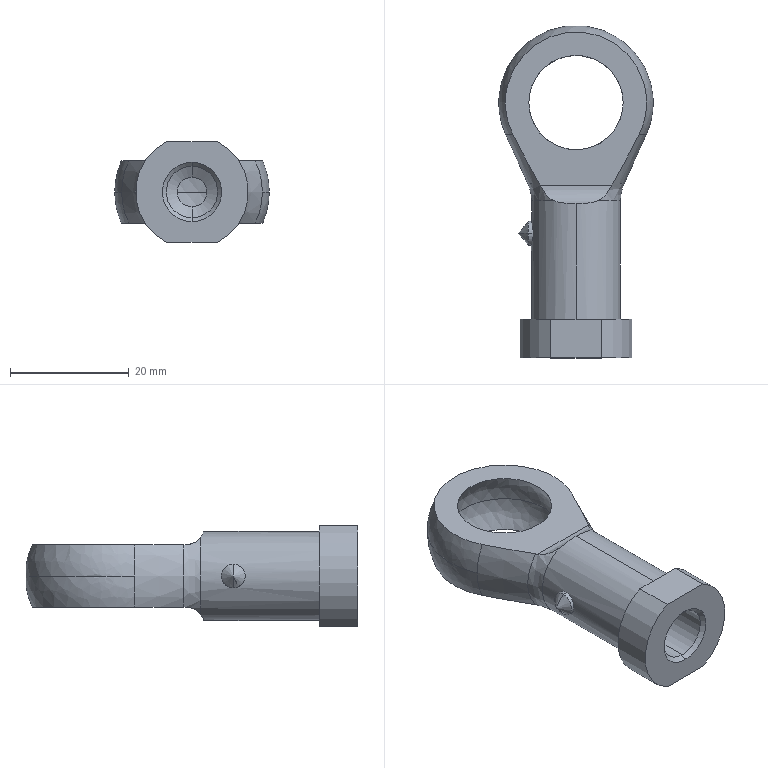Part | STEP file | 0229_Z_PHSC10A_1 | 1 solid | 32 faces | volume 7061 mm3 | cylinder 12 | cone 8 | spline 6 | plane 6 | commonest cylinder face diameters 4 x2 5 x2 6.5 x2 8.647 x2 15 x2 19 x2